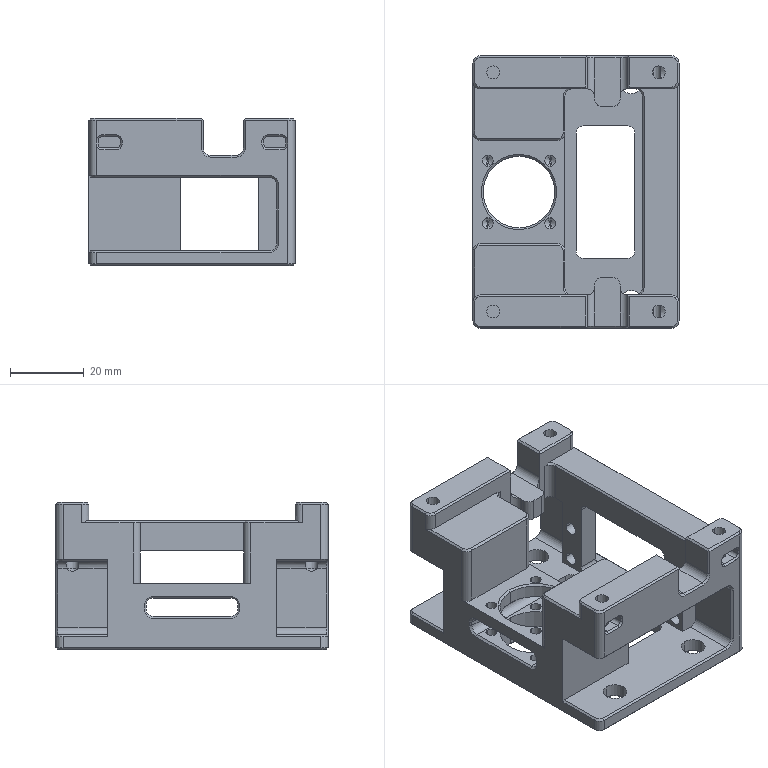NC program | Mastercam | posted with a generic post | part box 56 x 74 x 40 mm
Lines 1579 to 2693 of 45205:
(12 FEM |TOOL - 12|DIA. OFF. - 12|LEN. - 12|TOOL DIA. - 12.)
N3214 T12 M6
N3216 G0 G54 G90 X-50.6 Y28.398 C0. B0. S7000 M3
N3218 G43 H12 Z56.
N3220 Z8.
N3222 G1 Z5.513 F600.
N3224 X43.4 F3000.
N3226 G2 X47.457 Y24.341 J-4.057
N3228 X43.4 Y20.284 I-4.057
N3230 G1 X-43.4
N3232 G3 X-47.457 Y16.227 J-4.057
N3234 X-43.4 Y12.171 I4.057
N3236 G1 X43.4
N3238 G2 X47.457 Y8.114 J-4.057
N3240 X43.4 Y4.057 I-4.057
N3242 G1 X-43.4
N3244 G3 X-47.457 Y0. J-4.057
N3246 X-43.4 Y-4.057 I4.057
N3248 G1 X43.4
N3250 G2 X47.457 Y-8.114 J-4.057
N3252 X43.4 Y-12.171 I-4.057
N3254 G1 X-43.4
N3256 G3 X-47.456 Y-16.227 J-4.056
N3258 X-43.4 Y-20.284 I4.056
N3260 G1 X43.4
N3262 G2 X47.457 Y-24.341 J-4.057
N3264 X43.4 Y-28.398 I-4.057
N3266 G1 X-50.6
N3268 G0 Z55.513
N3270 Y28.398
N3272 Z7.513
N3274 G1 Z5.025 F600.
N3276 X43.4 F3000.
N3278 G2 X47.457 Y24.341 J-4.057
N3280 X43.4 Y20.284 I-4.057
N3282 G1 X-43.4
N3284 G3 X-47.457 Y16.227 J-4.057
N3286 X-43.4 Y12.171 I4.057
N3288 G1 X43.4
N3290 G2 X47.457 Y8.114 J-4.057
N3292 X43.4 Y4.057 I-4.057
N3294 G1 X-43.4
N3296 G3 X-47.457 Y0. J-4.057
N3298 X-43.4 Y-4.057 I4.057
N3300 G1 X43.4
N3302 G2 X47.457 Y-8.114 J-4.057
N3304 X43.4 Y-12.171 I-4.057
N3306 G1 X-43.4
N3308 G3 X-47.456 Y-16.227 J-4.056
N3310 X-43.4 Y-20.284 I4.056
N3312 G1 X43.4
N3314 G2 X47.457 Y-24.341 J-4.057
N3316 X43.4 Y-28.398 I-4.057
N3318 G1 X-50.6
N3320 G0 Z55.025
N3322 Y28.398
N3324 Z7.025
N3326 G1 Z4.537 F600.
N3328 X43.4 F3000.
N3330 G2 X47.457 Y24.341 J-4.057
N3332 X43.4 Y20.284 I-4.057
N3334 G1 X-43.4
N3336 G3 X-47.457 Y16.227 J-4.057
N3338 X-43.4 Y12.171 I4.057
N3340 G1 X43.4
N3342 G2 X47.457 Y8.114 J-4.057
N3344 X43.4 Y4.057 I-4.057
N3346 G1 X-43.4
N3348 G3 X-47.457 Y0. J-4.057
N3350 X-43.4 Y-4.057 I4.057
N3352 G1 X43.4
N3354 G2 X47.457 Y-8.114 J-4.057
N3356 X43.4 Y-12.171 I-4.057
N3358 G1 X-43.4
N3360 G3 X-47.456 Y-16.227 J-4.056
N3362 X-43.4 Y-20.284 I4.056
N3364 G1 X43.4
N3366 G2 X47.457 Y-24.341 J-4.057
N3368 X43.4 Y-28.398 I-4.057
N3370 G1 X-50.6
N3372 G0 Z54.538
N3374 Y28.398
N3376 Z6.537
N3378 G1 Z4.05 F600.
N3380 X43.4 F3000.
N3382 G2 X47.457 Y24.341 J-4.057
N3384 X43.4 Y20.284 I-4.057
N3386 G1 X-43.4
N3388 G3 X-47.457 Y16.227 J-4.057
N3390 X-43.4 Y12.171 I4.057
N3392 G1 X43.4
N3394 G2 X47.457 Y8.114 J-4.057
N3396 X43.4 Y4.057 I-4.057
N3398 G1 X-43.4
N3400 G3 X-47.457 Y0. J-4.057
N3402 X-43.4 Y-4.057 I4.057
N3404 G1 X43.4
N3406 G2 X47.457 Y-8.114 J-4.057
N3408 X43.4 Y-12.171 I-4.057
N3410 G1 X-43.4
N3412 G3 X-47.456 Y-16.227 J-4.056
N3414 X-43.4 Y-20.284 I4.056
N3416 G1 X43.4
N3418 G2 X47.457 Y-24.341 J-4.057
N3420 X43.4 Y-28.398 I-4.057
N3422 G1 X-50.6
N3424 G0 Z54.05
N3426 Y28.398
N3428 Z6.05
N3430 G1 Z3.563 F600.
N3432 X43.4 F3000.
N3434 G2 X47.457 Y24.341 J-4.057
N3436 X43.4 Y20.284 I-4.057
N3438 G1 X-43.4
N3440 G3 X-47.457 Y16.227 J-4.057
N3442 X-43.4 Y12.171 I4.057
N3444 G1 X43.4
N3446 G2 X47.457 Y8.114 J-4.057
N3448 X43.4 Y4.057 I-4.057
N3450 G1 X-43.4
N3452 G3 X-47.457 Y0. J-4.057
N3454 X-43.4 Y-4.057 I4.057
N3456 G1 X43.4
N3458 G2 X47.457 Y-8.114 J-4.057
N3460 X43.4 Y-12.171 I-4.057
N3462 G1 X-43.4
N3464 G3 X-47.456 Y-16.227 J-4.056
N3466 X-43.4 Y-20.284 I4.056
N3468 G1 X43.4
N3470 G2 X47.457 Y-24.341 J-4.057
N3472 X43.4 Y-28.398 I-4.057
N3474 G1 X-50.6
N3476 G0 Z53.563
N3478 Y28.398
N3480 Z5.563
N3482 G1 Z3.075 F600.
N3484 X43.4 F3000.
N3486 G2 X47.457 Y24.341 J-4.057
N3488 X43.4 Y20.284 I-4.057
N3490 G1 X-43.4
N3492 G3 X-47.457 Y16.227 J-4.057
N3494 X-43.4 Y12.171 I4.057
N3496 G1 X43.4
N3498 G2 X47.457 Y8.114 J-4.057
N3500 X43.4 Y4.057 I-4.057
N3502 G1 X-43.4
N3504 G3 X-47.457 Y0. J-4.057
N3506 X-43.4 Y-4.057 I4.057
N3508 G1 X43.4
N3510 G2 X47.457 Y-8.114 J-4.057
N3512 X43.4 Y-12.171 I-4.057
N3514 G1 X-43.4
N3516 G3 X-47.456 Y-16.227 J-4.056
N3518 X-43.4 Y-20.284 I4.056
N3520 G1 X43.4
N3522 G2 X47.457 Y-24.341 J-4.057
N3524 X43.4 Y-28.398 I-4.057
N3526 G1 X-50.6
N3528 G0 Z53.075
N3530 Y28.398
N3532 Z5.075
N3534 G1 Z2.587 F600.
N3536 X43.4 F3000.
N3538 G2 X47.457 Y24.341 J-4.057
N3540 X43.4 Y20.284 I-4.057
N3542 G1 X-43.4
N3544 G3 X-47.457 Y16.227 J-4.057
N3546 X-43.4 Y12.171 I4.057
N3548 G1 X43.4
N3550 G2 X47.457 Y8.114 J-4.057
N3552 X43.4 Y4.057 I-4.057
N3554 G1 X-43.4
N3556 G3 X-47.457 Y0. J-4.057
N3558 X-43.4 Y-4.057 I4.057
N3560 G1 X43.4
N3562 G2 X47.457 Y-8.114 J-4.057
N3564 X43.4 Y-12.171 I-4.057
N3566 G1 X-43.4
N3568 G3 X-47.456 Y-16.227 J-4.056
N3570 X-43.4 Y-20.284 I4.056
N3572 G1 X43.4
N3574 G2 X47.457 Y-24.341 J-4.057
N3576 X43.4 Y-28.398 I-4.057
N3578 G1 X-50.6
N3580 G0 Z52.587
N3582 Y28.398
N3584 Z4.588
N3586 G1 Z2.1 F600.
N3588 X43.4 F3000.
N3590 G2 X47.457 Y24.341 J-4.057
N3592 X43.4 Y20.284 I-4.057
N3594 G1 X-43.4
N3596 G3 X-47.457 Y16.227 J-4.057
N3598 X-43.4 Y12.171 I4.057
N3600 G1 X43.4
N3602 G2 X47.457 Y8.114 J-4.057
N3604 X43.4 Y4.057 I-4.057
N3606 G1 X-43.4
N3608 G3 X-47.457 Y0. J-4.057
N3610 X-43.4 Y-4.057 I4.057
N3612 G1 X43.4
N3614 G2 X47.457 Y-8.114 J-4.057
N3616 X43.4 Y-12.171 I-4.057
N3618 G1 X-43.4
N3620 G3 X-47.456 Y-16.227 J-4.056
N3622 X-43.4 Y-20.284 I4.056
N3624 G1 X43.4
N3626 G2 X47.457 Y-24.341 J-4.057
N3628 X43.4 Y-28.398 I-4.057
N3630 G1 X-50.6
N3632 G0 Z52.1
N3634 Y28.398
N3636 Z4.1
N3638 G1 Z1.613 F600.
N3640 X43.4 F3000.
N3642 G2 X47.457 Y24.341 J-4.057
N3644 X43.4 Y20.284 I-4.057
N3646 G1 X-43.4
N3648 G3 X-47.457 Y16.227 J-4.057
N3650 X-43.4 Y12.171 I4.057
N3652 G1 X43.4
N3654 G2 X47.457 Y8.114 J-4.057
N3656 X43.4 Y4.057 I-4.057
N3658 G1 X-43.4
N3660 G3 X-47.457 Y0. J-4.057
N3662 X-43.4 Y-4.057 I4.057
N3664 G1 X43.4
N3666 G2 X47.457 Y-8.114 J-4.057
N3668 X43.4 Y-12.171 I-4.057
N3670 G1 X-43.4
N3672 G3 X-47.456 Y-16.227 J-4.056
N3674 X-43.4 Y-20.284 I4.056
N3676 G1 X43.4
N3678 G2 X47.457 Y-24.341 J-4.057
N3680 X43.4 Y-28.398 I-4.057
N3682 G1 X-50.6
N3684 G0 Z51.612
N3686 Y28.398
N3688 Z3.612
N3690 G1 Z1.125 F600.
N3692 X43.4 F3000.
N3694 G2 X47.457 Y24.341 J-4.057
N3696 X43.4 Y20.284 I-4.057
N3698 G1 X-43.4
N3700 G3 X-47.457 Y16.227 J-4.057
N3702 X-43.4 Y12.171 I4.057
N3704 G1 X43.4
N3706 G2 X47.457 Y8.114 J-4.057
N3708 X43.4 Y4.057 I-4.057
N3710 G1 X-43.4
N3712 G3 X-47.457 Y0. J-4.057
N3714 X-43.4 Y-4.057 I4.057
N3716 G1 X43.4
N3718 G2 X47.457 Y-8.114 J-4.057
N3720 X43.4 Y-12.171 I-4.057
N3722 G1 X-43.4
N3724 G3 X-47.456 Y-16.227 J-4.056
N3726 X-43.4 Y-20.284 I4.056
N3728 G1 X43.4
N3730 G2 X47.457 Y-24.341 J-4.057
N3732 X43.4 Y-28.398 I-4.057
N3734 G1 X-50.6
N3736 G0 Z51.125
N3738 Y28.398
N3740 Z3.125
N3742 G1 Z.637 F600.
N3744 X43.4 F3000.
N3746 G2 X47.457 Y24.341 J-4.057
N3748 X43.4 Y20.284 I-4.057
N3750 G1 X-43.4
N3752 G3 X-47.457 Y16.227 J-4.057
N3754 X-43.4 Y12.171 I4.057
N3756 G1 X43.4
N3758 G2 X47.457 Y8.114 J-4.057
N3760 X43.4 Y4.057 I-4.057
N3762 G1 X-43.4
N3764 G3 X-47.457 Y0. J-4.057
N3766 X-43.4 Y-4.057 I4.057
N3768 G1 X43.4
N3770 G2 X47.457 Y-8.114 J-4.057
N3772 X43.4 Y-12.171 I-4.057
N3774 G1 X-43.4
N3776 G3 X-47.456 Y-16.227 J-4.056
N3778 X-43.4 Y-20.284 I4.056
N3780 G1 X43.4
N3782 G2 X47.457 Y-24.341 J-4.057
N3784 X43.4 Y-28.398 I-4.057
N3786 G1 X-50.6
N3788 G0 Z50.638
N3790 Y28.398
N3792 Z2.638
N3794 G1 Z.15 F600.
N3796 X43.4 F3000.
N3798 G2 X47.457 Y24.341 J-4.057
N3800 X43.4 Y20.284 I-4.057
N3802 G1 X-43.4
N3804 G3 X-47.457 Y16.227 J-4.057
N3806 X-43.4 Y12.171 I4.057
N3808 G1 X43.4
N3810 G2 X47.457 Y8.114 J-4.057
N3812 X43.4 Y4.057 I-4.057
N3814 G1 X-43.4
N3816 G3 X-47.457 Y0. J-4.057
N3818 X-43.4 Y-4.057 I4.057
N3820 G1 X43.4
N3822 G2 X47.457 Y-8.114 J-4.057
N3824 X43.4 Y-12.171 I-4.057
N3826 G1 X-43.4
N3828 G3 X-47.456 Y-16.227 J-4.056
N3830 X-43.4 Y-20.284 I4.056
N3832 G1 X43.4
N3834 G2 X47.457 Y-24.341 J-4.057
N3836 X43.4 Y-28.398 I-4.057
N3838 G1 X-50.6
N3840 G0 Z50.15
N3842 M5
N3844 G0 G28 G91 Z0.
N3846 G28
N3848 M01
N3850 G0 G17 G40 G80 G90 G94 G98
N3852 G0 G28 G91 Z0.
(100 FEM |TOOL - 24|DIA. OFF. - 24|LEN. - 24|TOOL DIA. - 100.)
N3854 T24 M6
N3856 G0 G54 G90 X-121. Y0. C0. B0. S4000 M3
N3858 G43 H24 Z56.
N3860 Z8.
N3862 G1 Z0. F600.
N3864 X121. F1000.
N3866 G0 Z50.
N3868 M5
N3870 G0 G28 G91 Z0.
N3872 G28
N3874 M01
N3876 G0 G17 G40 G80 G90 G94 G98
N3878 G0 G28 G91 Z0.
(4 CHM |TOOL - 5|DIA. OFF. - 5|LEN. - 5|TOOL DIA. - 4.)
N3880 T5 M6
N3882 G0 G54 G90 X35.4 Y-29.45 C0. B0. S6000 M3
N3884 G43 H5 Z50.
N3886 Z1.
N3888 G1 Z-1. F600.
N3890 Y-29.05 F1000.
N3892 G3 X35. Y-28.65 I-.4
N3894 G1 X-35.
N3896 G2 X-37.65 Y-26. J2.65
N3898 G1 Y26.
N3900 G2 X-35. Y28.65 I2.65
N3902 G1 X35.
N3904 G2 X37.65 Y26. J-2.65
N3906 G1 Y-26.
N3908 G2 X35. Y-28.65 I-2.65
N3910 G1 X34.5
N3912 G3 X34.1 Y-29.05 J-.4
N3914 G1 Y-29.45
N3916 G0 Z50.
N3918 M5
N3920 G0 G28 G91 Z0.
N3922 G28
N3924 M01
N3926 G0 G17 G40 G80 G90 G94 G98
N3928 G0 G28 G91 Z0.
(8 FEM |TOOL - 8|DIA. OFF. - 8|LEN. - 8|TOOL DIA. - 8.)
N3930 T8 M6
N3932 G0 G54 G90 X-6.691 Y16.106 C0. B0. S7000 M3
N3934 G43 H8 Z50.
N3936 Z6.27
N3938 G1 Z5.77 F600.
N3940 X-6.702 Z5.561 F3000.
N3942 X-6.734 Z5.354
N3944 X-6.788 Z5.152
N3946 X-6.863 Z4.956
N3948 X-6.959 Z4.77
N3950 X-7.073 Z4.594
N3952 X-7.204 Z4.431
N3954 X-7.352 Z4.283
N3956 X-7.515 Z4.152
N3958 X-7.691 Z4.038
N3960 X-7.877 Z3.943
N3962 X-8.073 Z3.868
N3964 X-8.275 Z3.813
N3966 X-8.482 Z3.781
N3968 X-8.691 Z3.77
N3970 G3 X-18.691 Y6.106 Z1. J-10.
N3972 G1 Y2.309 Z.935
N3974 X-16.468 Z.925
N3976 X-12.068 Z.85
N3978 X-11.724 Z.844
N3980 X-7.668 Z.775
N3982 X-3.268 Z.7
N3984 X1.132 Z.625
N3986 X5.532 Z.55
N3988 X9.932 Z.475
N3990 X14.332 Z.4
N3992 X18.691 Z.326
N3994 Y2.913 Z.325
N3996 Y6.691 Z.261
N3998 X16.435 Z.25
N4000 X12.035 Z.175
N4002 X7.635 Z.1
N4004 X3.235 Z.025
N4006 X0. Z-.03
N4008 X-1.165 Z-.05
N4010 X-5.565 Z-.125
N4012 X-9.965 Z-.2
N4014 X-14.365 Z-.275
N4016 X-18.691 Z-.349
N4018 Y5.883 Z-.35
N4020 Y2.309 Z-.411
N4022 X-16.124 Z-.425
N4024 X-11.724 Z-.5
N4026 X18.691
N4028 Y6.691
N4030 X0.
N4032 X-18.691
N4034 Y2.309
N4036 X-11.724
N4038 G2 X-10.919 Y1.662 J-.825
N4040 G1 X-10.055 Y-2.253
N4042 G3 X-9.249 Y-2.9 I.806 J.178
N4044 G1 X23.9
N4046 Y11.9
N4048 X0.
N4050 X-23.9
N4052 Y-2.9
N4054 X-9.249
N4056 G3 X-8.667 Y-2.659 J.825
N4058 G1 X-.697 Y5.281
N4060 G3 X-.454 Y5.866 I-.583 J.585
N4062 X-1.28 Y6.691 I-.826
N4064 G1 X-5.68 Z-.571
N4066 X-10.08 Z-.643
N4068 X-14.48 Z-.714
N4070 X-18.691 Z-.783
N4072 Y5.415 Z-.786
N4074 Y2.309 Z-.836
N4076 X-15.574 Z-.857
N4078 X-11.174 Z-.929
N4080 X-6.774 Z-1.
N4082 X0.
N4084 X18.691
N4086 Y6.691
N4088 X-18.691
N4090 Y2.309
N4092 X-6.774
N4094 G2 X-5.969 Y1.662 J-.825
N4096 G1 X-5.105 Y-2.253
N4098 G3 X-4.299 Y-2.9 I.806 J.178
N4100 G1 X0.
N4102 X23.9
N4104 Y11.9
N4106 X-23.9
N4108 Y-2.9
N4110 X-4.299
N4112 G3 X-3.474 Y-2.075 J.825
N4114 X-3.491 Y-1.907 I-.825
N4116 G1 X-5.138 Y6.033
N4118 G3 X-5.946 Y6.691 I-.808 J-.167
N4120 G1 X-10.346 Z-1.071
N4122 X-14.746 Z-1.143
N4124 X-18.691 Z-1.207
N4126 Y4.742 Z-1.214
N4128 Y2.309 Z-1.254
N4130 X-15.024 Z-1.286
N4132 X-10.624 Z-1.357
N4134 X-6.224 Z-1.429
N4136 X-1.824 Z-1.5
N4138 X0.
N4140 X18.691
N4142 Y6.691
N4144 X-18.691
N4146 Y2.309
N4148 X-1.824
N4150 G2 X-1. Y1.524 J-.825
N4152 G1 X-.824 Y-2.115
N4154 G3 X0. Y-2.9 I.824 J.04
N4156 G1 X23.9
N4158 Y11.9
N4160 X-23.9
N4162 Y-2.9
N4164 X0.
N4166 G3 X.825 Y-2.075 J.825
N4168 X.504 Y-1.422 I-.825
N4170 G1 X-9.773 Y6.519
N4172 G3 X-10.277 Y6.691 I-.504 J-.653
N4174 G1 X-14.677 Z-1.571
N4176 X-18.691 Z-1.637
N4178 Y4.887 Z-1.643
N4180 Y2.309 Z-1.685
N4182 X-15.125 Z-1.714
N4184 X-10.725 Z-1.786
N4186 X-6.325 Z-1.857
N4188 X-1.925 Z-1.929
N4190 X0. Z-1.96
N4192 X2.475 Z-2.
N4194 X18.691
N4196 Y6.691
N4198 X-18.691
N4200 Y2.309
N4202 X0.
N4204 X2.475
N4206 G2 X3.281 Y1.662 J-.825
N4208 G1 X4.144 Y-2.253
N4210 G3 X4.95 Y-2.9 I.806 J.178
N4212 G1 X23.9
N4214 Y11.9
N4216 X-23.9
N4218 Y-2.9
N4220 X0.
N4222 X4.95
N4224 G3 X5.775 Y-2.075 J.825
N4226 X5.251 Y-1.307 I-.825
N4228 G1 X-15.017 Y6.634
N4230 G3 X-15.318 Y6.691 I-.301 J-.768
N4232 G1 X-18.691 Z-2.055
N4234 Y3.865 Z-2.071
N4236 Y2.309 Z-2.097
N4238 X-14.575 Z-2.143
N4240 X-10.175 Z-2.214
N4242 X-5.775 Z-2.286
N4244 X-1.375 Z-2.357
N4246 X0. Z-2.379
N4248 X3.025 Z-2.429
N4250 X7.425 Z-2.5
N4252 X18.691
N4254 Y6.691
N4256 X-18.691
N4258 Y2.309
N4260 X0.
N4262 X7.425
N4264 G2 X8.231 Y1.662 J-.825
N4266 G1 X9.094 Y-2.253
N4268 G3 X9.9 Y-2.9 I.806 J.178
N4270 G1 X23.9
N4272 Y11.9
N4274 X-23.9
N4276 Y-2.9
N4278 X0.
N4280 X9.9
N4282 G3 X10.725 Y-2.103 J.825
N4284 G1 Y-2.075
N4286 G3 X9.955 Y-1.252 I-.825
N4288 G1 X-18.48 Y.661
N4290 G2 X-19.25 Y1.484 I.055 J.823
N4292 G1 Y1.512
N4294 G2 X-18.425 Y2.309 I.825 J-.028
N4296 G1 X-14.025 Z-2.571
N4298 X-9.625 Z-2.643
N4300 X-5.225 Z-2.714
N4302 X-.825 Z-2.786
N4304 X0. Z-2.799
N4306 X3.575 Z-2.857
N4308 X7.975 Z-2.929
N4310 X12.375 Z-3.
N4312 X18.691
N4314 Y6.691
N4316 X-18.691
N4318 Y2.309
N4320 X0.
N4322 X12.375
N4324 G2 X13.181 Y1.662 J-.825
N4326 G1 X14.044 Y-2.253
N4328 G3 X14.85 Y-2.9 I.806 J.178
N4330 G1 X23.9
N4332 Y11.9
N4334 X-23.9
N4336 Y-2.9
N4338 X0.
N4340 X14.85
N4342 G3 X15.675 Y-2.103 J.825
N4344 G1 Y-2.075
N4346 G3 X14.905 Y-1.252 I-.825
N4348 G1 X-13.53 Y.661
N4350 G2 X-14.3 Y1.484 I.055 J.823
N4352 G1 Y1.512
N4354 G2 X-13.475 Y2.309 I.825 J-.028
N4356 G1 X-9.075 Z-3.071
N4358 X-4.675 Z-3.143
N4360 X-.275 Z-3.214
N4362 X0. Z-3.219
N4364 X4.125 Z-3.286
N4366 X8.525 Z-3.357
N4368 X12.925 Z-3.429
N4370 X17.325 Z-3.5
N4372 X18.691
N4374 Y6.691
N4376 X-18.691
N4378 Y2.309
N4380 X0.
N4382 X17.325
N4384 G2 X18.131 Y1.662 J-.825
N4386 G1 X18.994 Y-2.253
N4388 G3 X19.8 Y-2.9 I.806 J.178
N4390 G1 X23.9
N4392 Y11.9
N4394 X-23.9
N4396 Y-2.9
N4398 X0.
N4400 X19.8
N4402 G3 X20.624 Y-2.104 J.825
N4404 X20.625 Y-2.075 I-.824 J.029
N4406 X19.859 Y-1.252 I-.825
N4408 G1 X-7.006 Y.661
N4410 G2 X-7.772 Y1.484 I.059 J.823
N4412 G1 Y1.513
N4414 G2 X-6.947 Y2.309 I.825 J-.029
N4416 G1 X-2.547 Z-3.566
N4418 X0. Z-3.605
N4420 X1.853 Z-3.632
N4422 X6.253 Z-3.699
N4424 X10.653 Z-3.765
N4426 X15.053 Z-3.831
N4428 X18.691 Z-3.886
N4430 Y4.784 Z-3.897
N4432 Y6.691
N4434 X-18.691
N4436 Y2.309
N4438 X0.
N4440 X18.691
N4442 Y4.784
N4444 G2 X19.338 Y5.59 I.825
N4446 G1 X23.252 Y6.453
N4448 G3 X23.9 Y7.259 I-.177 J.806
N4450 G1 Y11.9
N4452 X-23.9
N4454 Y-2.9
N4456 X0.
N4458 X23.9
N4460 Y7.259
N4462 G3 X23.08 Y8.084 I-.825
N4464 G1 X13.178 Y8.147
N4466 G2 X12.359 Y8.972 I.006 J.825
N4468 G1 Y11.9 Z-3.932
N4470 X9.074 Z-3.949
N4472 X4.674 Z-4.
N4474 G3 X3.849 Y11.075 J-.825
N4476 X3.943 Y10.692 I.825
N4478 G1 X5.405 Y7.898
N4480 G2 X5.499 Y7.515 I-.731 J-.383
N4482 X4.674 Y6.69 I-.825
N4484 G1 X-7.149
N4486 Y2.309
N4488 X0.
N4490 X7.149
N4492 Y6.691
N4494 X4.674 Y6.69
N4496 G2 X3.869 Y7.338 J.825
N4498 G1 X3.005 Y11.252
N4500 G3 X2.199 Y11.9 I-.806 J-.177
N4502 G1 X-12.359 Y11.899
N4504 Y-2.9
N4506 X0.
N4508 X12.359
N4510 Y11.9
N4512 X2.199
N4514 G3 X1.374 Y11.075 J-.825
N4516 X1.386 Y10.935 I.825
N4518 G1 X3.644 Y-2.215
N4520 G3 X4.457 Y-2.9 I.813 J.14
N4522 G1 X8.857 Z-4.071
N4524 X11.9 Z-4.121
N4526 Y.278 Z-4.143
N4528 Y4.678 Z-4.214
N4530 Y9.078 Z-4.286
N4532 Y11.9 Z-4.332
N4534 X8.524 Z-4.357
N4536 X4.124 Z-4.429
N4538 X-.276 Z-4.5
N4540 G3 X-1.101 Y11.075 J-.825
N4542 X-1.007 Y10.693 I.825
N4544 G1 X.455 Y7.898
N4546 G2 X.549 Y7.516 I-.731 J-.382
N4548 X-.276 Y6.691 I-.825
N4550 G1 X-6.691
N4552 Y2.309
N4554 X0.
N4556 X6.691
N4558 Y6.691
N4560 X-.276
N4562 G2 X-1.081 Y7.338 J.825
N4564 G1 X-1.945 Y11.253
N4566 G3 X-2.751 Y11.9 I-.806 J-.178
N4568 G1 X-11.9
N4570 Y-2.9
N4572 X0.
N4574 X11.9
N4576 Y11.9
N4578 X-2.751
N4580 G3 X-3.576 Y11.075 J-.825
N4582 X-3.341 Y10.498 I.825
N4584 G1 X9.505 Y-2.652
N4586 G3 X10.095 Y-2.9 I.59 J.577
N4588 G1 X11.9 Z-4.529
N4590 Y1.113 Z-4.571
N4592 Y5.513 Z-4.643
N4594 Y9.913 Z-4.714
N4596 Y11.9 Z-4.747
N4598 X7.974 Z-4.786
N4600 X3.574 Z-4.857
N4602 X-.826 Z-4.929
N4604 X-5.226 Z-5.
N4606 G3 X-6.051 Y11.075 J-.825
N4608 X-5.957 Y10.693 I.825
N4610 G1 X-4.495 Y7.898
N4612 G2 X-4.401 Y7.516 I-.731 J-.382
N4614 X-5.226 Y6.691 I-.825
N4616 G1 X-6.691
N4618 Y2.309
N4620 X0.
N4622 X6.691
N4624 Y6.691
N4626 X-5.226
N4628 G2 X-6.031 Y7.338 J.825
N4630 G1 X-6.895 Y11.253
N4632 G3 X-7.701 Y11.9 I-.806 J-.178
N4634 G1 X-11.9
N4636 Y-2.9
N4638 X0.
N4640 X11.9
N4642 Y11.9
N4644 X-7.701
N4646 G3 X-8.526 Y11.075 J-.825
N4648 X-7.793 Y10.255 I.825
N4650 G1 X10.982 Y8.138
N4652 G3 X11.075 Y8.133 I.093 J.82
N4654 X11.9 Y8.958 J.825
N4656 G1 Y11.9 Z-5.048
N4658 X8.628 Z-5.071
N4660 X4.228 Z-5.143
N4662 X-.172 Z-5.214
N4664 X-4.572 Z-5.286
N4666 X-8.972 Z-5.357
N4668 X-11.9 Z-5.405
N4670 Y8.616 Z-5.429
N4672 Y4.216 Z-5.5
N4674 G3 X-11.075 Y3.391 I.825
N4676 X-10.692 Y3.485 J.825
N4678 G1 X-7.898 Y4.947
N4680 G2 X-7.516 Y5.041 I.382 J-.731
N4682 X-6.691 Y4.216 J-.825
N4684 G1 Y2.309
N4686 X0.
N4688 X6.691
N4690 Y6.691
N4692 X-6.691
N4694 Y4.216
N4696 G2 X-7.338 Y3.41 I-.825
N4698 G1 X-11.253 Y2.547
N4700 G3 X-11.9 Y1.741 I.178 J-.806
N4702 G1 Y-2.9
N4704 X0.
N4706 X11.9
N4708 Y11.9
N4710 X-11.9
N4712 Y1.741
N4714 G3 X-11.075 Y.916 I.825
N4716 X-10.545 Y1.109 J.825
N4718 G1 X.581 Y10.443
N4720 G3 X.875 Y11.075 I-.531 J.632
N4722 X.05 Y11.9 I-.825
N4724 G1 X-4.35 Z-5.571
N4726 X-8.75 Z-5.643
N4728 X-11.9 Z-5.694
N4730 Y8.828 Z-5.714
N4732 Y4.428 Z-5.786
N4734 Y.028 Z-5.857
N4736 Y-2.9 Z-5.905
N4738 X-8.616 Z-5.929
N4740 X-4.216 Z-6.
N4742 G3 X-3.391 Y-2.075 J.825
N4744 X-3.485 Y-1.693 I-.825
N4746 G1 X-4.947 Y1.102
N4748 G2 X-5.041 Y1.484 I.731 J.382
N4750 X-4.216 Y2.309 I.825
N4752 G1 X0.
N4754 X6.691
N4756 Y6.691
N4758 X-6.691
N4760 Y2.309
N4762 X-4.216
N4764 G2 X-3.41 Y1.662 J-.825
N4766 G1 X-2.546 Y-2.253
N4768 G3 X-1.741 Y-2.9 I.805 J.178
N4770 G1 X0.
N4772 X11.9
N4774 Y11.9
N4776 X-11.9
N4778 Y-2.9
N4780 X-1.741
N4782 G3 X-.916 Y-2.075 J.825
N4784 X-.93 Y-1.925 I-.825
N4786 G1 X-3.36 Y11.225
N4788 G3 X-4.171 Y11.9 I-.811 J-.15
N4790 G1 X-8.571 Z-6.071
N4792 X-11.9 Z-6.125
N4794 Y9.023 Z-6.143
N4796 Y4.623 Z-6.214
N4798 Y.223 Z-6.286
N4800 Y-2.9 Z-6.336
N4802 X-8.8 Z-6.357
N4804 X-4.4 Z-6.429
N4806 X0. Z-6.5
N4808 G3 X.825 Y-2.075 J.825
N4810 X.731 Y-1.693 I-.825
N4812 G1 X-.731 Y1.102
N4814 G2 X-.825 Y1.484 I.731 J.382
N4816 X0. Y2.309 I.825
N4818 G1 X6.691
N4820 Y6.691
N4822 X-6.691
N4824 Y2.309
N4826 X0.
N4828 G2 X.806 Y1.662 J-.825
N4830 G1 X1.669 Y-2.253
N4832 G3 X2.475 Y-2.9 I.806 J.178
N4834 G1 X11.9
N4836 Y11.9
N4838 X-11.9
N4840 Y-2.9
N4842 X0.
N4844 X2.475
N4846 G3 X3.3 Y-2.075 J.825
N4848 X3.09 Y-1.525 I-.825
N4850 G1 X-8.676 Y11.625
N4852 G3 X-9.291 Y11.9 I-.615 J-.55
N4854 G1 X-11.9 Z-6.542
N4856 Y8.357 Z-6.571
N4858 Y3.957 Z-6.643
N4860 Y-.443 Z-6.714
N4862 Y-2.9 Z-6.754
N4864 X-8.25 Z-6.786
N4866 X-3.85 Z-6.857
N4868 X0. Z-6.92
N4870 X.55 Z-6.929
N4872 X4.95 Z-7.
N4874 G3 X5.775 Y-2.075 J.825
N4876 X5.681 Y-1.693 I-.825
N4878 G1 X4.219 Y1.102
N4880 G2 X4.125 Y1.484 I.731 J.382
N4882 X4.95 Y2.309 I.825
N4884 G1 X6.691
N4886 Y6.691
N4888 X-6.691
N4890 Y2.309
N4892 X0.
N4894 X4.95
N4896 G2 X5.756 Y1.662 J-.825
N4898 G1 X6.619 Y-2.253
N4900 G3 X7.425 Y-2.9 I.806 J.178
N4902 G1 X11.9
N4904 Y11.9
N4906 X-11.9
N4908 Y-2.9
N4910 X0.
N4912 X7.425
N4914 G3 X8.25 Y-2.075 J.825
N4916 X7.519 Y-1.255 I-.825
N4918 G1 X-10.981 Y.862
N4920 G3 X-11.075 Y.867 I-.094 J-.82
N4922 X-11.9 Y.042 J-.825
N4924 G1 Y-2.9 Z-7.048
N4926 X-8.628 Z-7.071
N4928 X-4.228 Z-7.143
N4930 X0. Z-7.211
N4932 X.172 Z-7.214
N4934 X4.572 Z-7.286
N4936 X8.972 Z-7.357
N4938 X11.9 Z-7.405
N4940 Y.384 Z-7.429
N4942 Y4.784 Z-7.5
N4944 G3 X11.075 Y5.609 I-.825
N4946 X10.692 Y5.515 J-.825
N4948 G1 X7.898 Y4.053
N4950 G2 X7.516 Y3.959 I-.382 J.731
N4952 X6.691 Y4.784 J.825
N4954 G1 Y6.691
N4956 X-6.691
N4958 Y2.309
N4960 X0.
N4962 X6.691
N4964 Y4.784
N4966 G2 X7.338 Y5.59 I.825
N4968 G1 X11.253 Y6.453
N4970 G3 X11.9 Y7.259 I-.178 J.806
N4972 G1 Y11.9
N4974 X-11.9
N4976 Y-2.9
N4978 X0.
N4980 X11.9
N4982 Y7.259
N4984 G3 X11.075 Y8.084 I-.825
N4986 X10.545 Y7.891 J-.825
N4988 G1 X-.581 Y-1.443
N4990 G3 X-.875 Y-2.075 I.531 J-.632
N4992 X-.05 Y-2.9 I.825
N4994 G1 X0. Z-7.501
N4996 X4.35 Z-7.571
N4998 X8.75 Z-7.643
N5000 X11.9 Z-7.694
N5002 Y.172 Z-7.714
N5004 Y4.572 Z-7.786
N5006 Y8.972 Z-7.857
N5008 Y11.9 Z-7.905
N5010 X8.616 Z-7.929
N5012 X4.216 Z-8.
N5014 G3 X3.391 Y11.075 J-.825
N5016 X3.485 Y10.693 I.825
N5018 G1 X4.947 Y7.898
N5020 G2 X5.041 Y7.516 I-.731 J-.382
N5022 X4.216 Y6.691 I-.825
N5024 G1 X-6.691
N5026 Y2.309
N5028 X0.
N5030 X6.691
N5032 Y6.691
N5034 X4.216
N5036 G2 X3.41 Y7.338 J.825
N5038 G1 X2.546 Y11.253
N5040 G3 X1.741 Y11.9 I-.805 J-.178
N5042 G1 X-11.9
N5044 Y-2.9
N5046 X0.
N5048 X11.9
N5050 Y11.9
N5052 X1.741
N5054 G3 X.916 Y11.075 J-.825
N5056 X.945 Y10.856 I.825
N5058 G1 X4.559 Y-2.294
N5060 G3 X5.354 Y-2.9 I.795 J.219
N5062 G1 X9.754 Z-8.071
N5064 X11.9 Z-8.106
N5066 Y.941 Z-8.143
N5068 Y5.341 Z-8.214
N5070 Y9.741 Z-8.286
N5072 Y11.9 Z-8.321
N5074 X8.066 Z-8.357
N5076 X3.666 Z-8.429
N5078 X-.734 Z-8.5
N5080 G3 X-1.559 Y11.075 J-.825
N5082 X-1.465 Y10.693 I.825
N5084 G1 X-.003 Y7.898
N5086 G2 X.091 Y7.516 I-.731 J-.382
N5088 X-.734 Y6.691 I-.825
N5090 G1 X-6.691
N5092 Y2.309
N5094 X0.
N5096 X6.691
N5098 Y6.691
N5100 X-.734
N5102 G2 X-1.54 Y7.338 J.825
N5104 G1 X-2.404 Y11.253
N5106 G3 X-3.209 Y11.9 I-.805 J-.178
N5108 G1 X-11.9
N5110 Y-2.9
N5112 X0.
N5114 X11.9
N5116 Y11.9
N5118 X-3.209
N5120 G3 X-4.034 Y11.075 J-.825
N5122 X-3.759 Y10.459 I.825
N5124 G1 X10.526 Y-2.289
N5126 G3 X11.075 Y-2.498 I.549 J.615
N5128 X11.9 Y-1.674 J.824
N5130 G1 Y2.726 Z-8.571
N5132 Y7.126 Z-8.643
N5134 Y11.526 Z-8.714
N5136 Y11.9 Z-8.72
N5138 X7.516 Z-8.786
N5140 X3.116 Z-8.857
N5142 X-1.284 Z-8.929
N5144 X-5.684 Z-9.
N5146 G3 X-6.509 Y11.075 J-.825
N5148 X-6.415 Y10.693 I.825
N5150 G1 X-4.953 Y7.898
N5152 G2 X-4.859 Y7.516 I-.731 J-.382
N5154 X-5.684 Y6.691 I-.825
N5156 G1 X-6.691
N5158 Y2.309
N5160 X0.
N5162 X6.691
N5164 Y6.691
N5166 X-5.684
N5168 G2 X-6.49 Y7.338 J.825
N5170 G1 X-7.354 Y11.253
N5172 G3 X-8.159 Y11.9 I-.805 J-.178
N5174 G1 X-11.9
N5176 Y-2.9
N5178 X0.
N5180 X11.9
N5182 Y11.9
N5184 X-8.159
N5186 G3 X-8.983 Y11.12 J-.825
N5188 X-8.984 Y11.075 I.824 J-.045
N5190 X-8.249 Y10.255 I.825
N5192 G1 X10.985 Y8.138
N5194 G3 X11.075 Y8.133 I.09 J.82
N5196 X11.9 Y8.958 J.825
N5198 G1 Y11.9 Z-9.048
N5200 X8.628 Z-9.071
N5202 X4.228 Z-9.143
N5204 X-.172 Z-9.214
N5206 X-4.572 Z-9.286
N5208 X-8.972 Z-9.357
N5210 X-11.9 Z-9.405
N5212 Y8.616 Z-9.429
N5214 Y4.216 Z-9.5
N5216 G3 X-11.075 Y3.391 I.825
N5218 X-10.692 Y3.485 J.825
N5220 G1 X-7.898 Y4.947
N5222 G2 X-7.516 Y5.041 I.382 J-.731
N5224 X-6.691 Y4.216 J-.825
N5226 G1 Y2.309
N5228 X0.
N5230 X6.691
N5232 Y6.691
N5234 X-6.691
N5236 Y4.216
N5238 G2 X-7.338 Y3.41 I-.825
N5240 G1 X-11.253 Y2.547
N5242 G3 X-11.9 Y1.741 I.178 J-.806
N5244 G1 Y-2.9
N5246 X0.
N5248 X11.9
N5250 Y11.9
N5252 X-11.9
N5254 Y1.741
N5256 G3 X-11.075 Y.916 I.825
N5258 X-10.545 Y1.109 J.825
N5260 G1 X.581 Y10.443
N5262 G3 X.876 Y11.075 I-.53 J.632
N5264 X.051 Y11.9 I-.825
N5266 G1 X-4.349 Z-9.571
N5268 X-8.749 Z-9.643
N5270 X-11.9 Z-9.694
N5272 Y8.828 Z-9.714
N5274 Y4.428 Z-9.786
N5276 Y.028 Z-9.857
N5278 Y-2.9 Z-9.905
N5280 X-8.615 Z-9.929
N5282 X-4.215 Z-10.
N5284 G3 X-3.39 Y-2.075 J.825
N5286 X-3.484 Y-1.693 I-.825
N5288 G1 X-4.946 Y1.102
N5290 G2 X-5.04 Y1.484 I.731 J.382
N5292 X-4.215 Y2.309 I.825
N5294 G1 X0.
N5296 X6.69
N5298 Y6.691
N5300 X-6.69
N5302 Y2.309
N5304 X-4.215
N5306 G2 X-3.41 Y1.662 J-.825
N5308 G1 X-2.546 Y-2.253
N5310 G3 X-1.74 Y-2.9 I.806 J.178
N5312 G1 X0.
N5314 X11.9
N5316 Y11.9
N5318 X-11.9
N5320 Y-2.9
N5322 X-1.74
N5324 G3 X-.915 Y-2.075 J.825
N5326 X-.929 Y-1.925 I-.825
N5328 G1 X-3.359 Y11.225
N5330 G3 X-4.171 Y11.9 I-.812 J-.15
N5332 G1 X-8.571 Z-10.071
N5334 X-11.9 Z-10.125
N5336 Y9.023 Z-10.143
N5338 Y4.623 Z-10.214
N5340 Y.223 Z-10.286
N5342 Y-2.9 Z-10.336
N5344 X-8.8 Z-10.357
N5346 X-4.4 Z-10.429
N5348 X0. Z-10.5
N5350 G3 X.825 Y-2.075 J.825
N5352 X.731 Y-1.693 I-.825
N5354 G1 X-.731 Y1.102
N5356 G2 X-.825 Y1.484 I.731 J.382
N5358 X0. Y2.309 I.825
N5360 G1 X6.69
N5362 Y6.691
N5364 X-6.69
N5366 Y2.309
N5368 X0.
N5370 G2 X.806 Y1.662 J-.825
N5372 G1 X1.669 Y-2.253
N5374 G3 X2.475 Y-2.9 I.806 J.178
N5376 G1 X11.9
N5378 Y11.9
N5380 X-11.9
N5382 Y-2.9
N5384 X0.
N5386 X2.475
N5388 G3 X4.475 Y-.9 Z-9.946 J2.
N5390 G1 Y-.691 Z-9.935
N5392 Y-.484 Z-9.902
N5394 Y-.282 Z-9.848
N5396 Y-.087 Z-9.773
N5398 Y.1 Z-9.678
N5400 Y.276 Z-9.564
N5402 Y.438 Z-9.432
N5404 Y.586 Z-9.284
N5406 Y.718 Z-9.122
N5408 Y.832 Z-8.946
N5410 Y.927 Z-8.76
N5412 Y1.002 Z-8.564
N5414 Y1.056 Z-8.362
N5416 Y1.089 Z-8.155
N5418 Y1.1 Z-7.946
N5420 Z-7.446
N5422 G0 Z50.
N5424 M5
N5426 G0 G28 G91 Z0.
N5428 G28
N5430 M01
N5432 G0 G17 G40 G80 G90 G94 G98
N5434 G0 G28 G91 Z0.